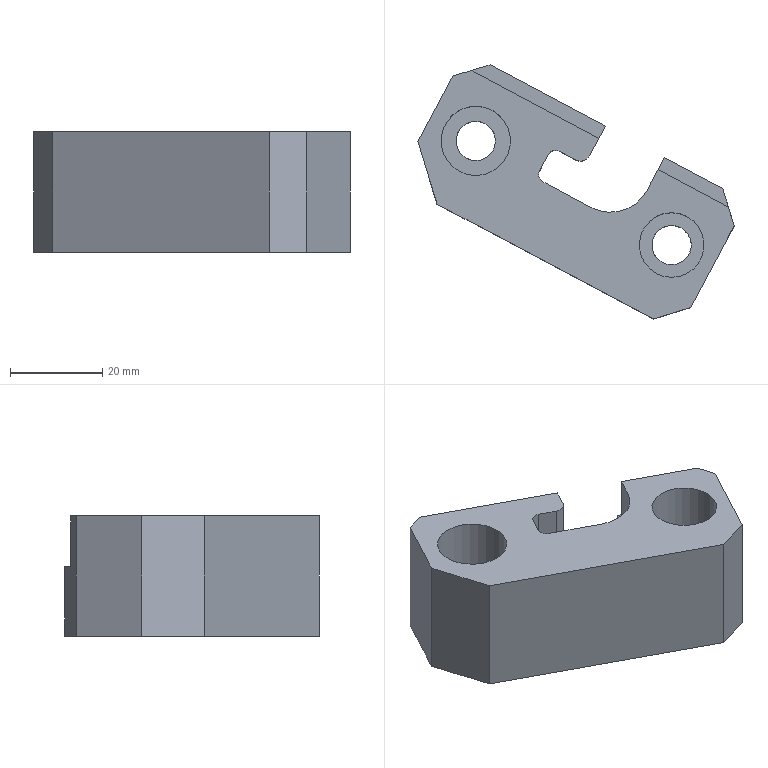Part | STEP file | gslz 2016.10.28-13_id1670_x_t | 1 solid | 34 faces | box 68.435 x 55.014 x 26 mm | volume 39925 mm3 | plane 24 | cylinder 10 | commonest cylinder face diameters 3.5 x2 8.5 x2 10 x2 4.5 x1 14 x1 15 x1